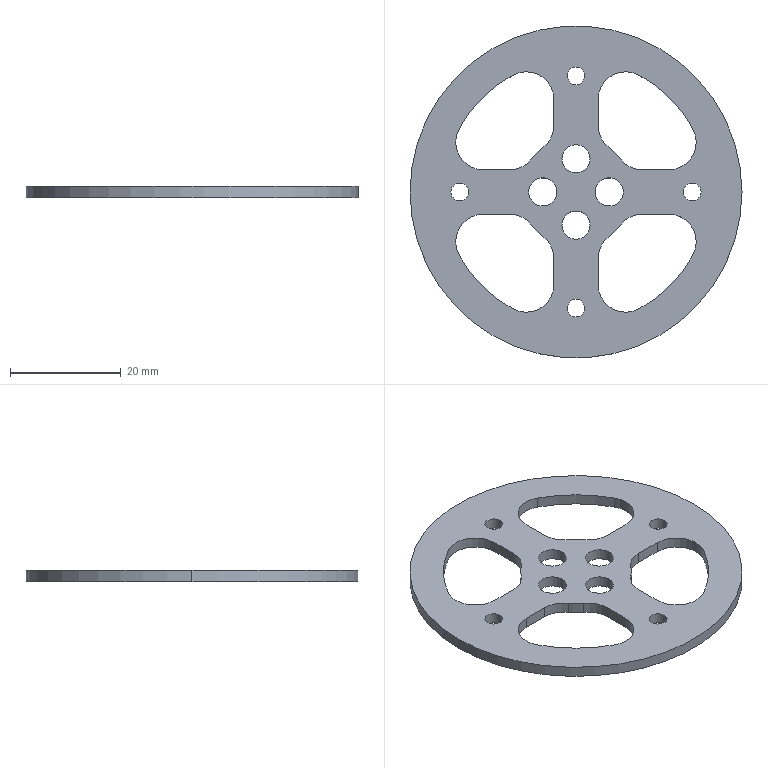Part | SolidWorks | features ICE 2, Extrusion 1 | 1 solid | 54 faces | box 60 x 60 x 2 mm | volume 3559 mm3 | cylinder 44 | plane 10 | commonest cylinder face diameters 10 x18 3.2 x8 5.1 x8 20 x4 48 x4 60 x2